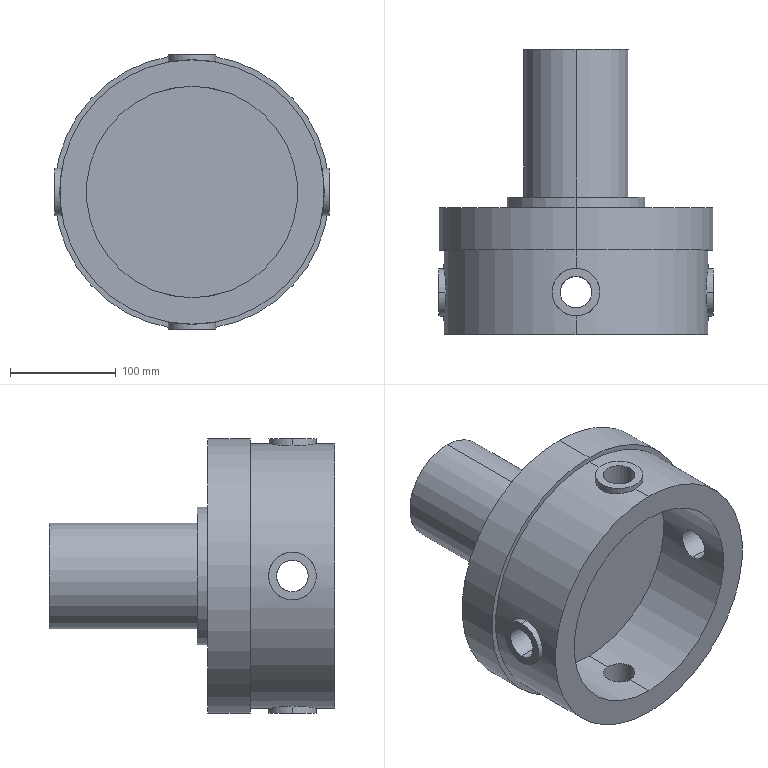Part | SolidWorks | features ICE 5, CirPattern 2, Extrusion 1 | 1 solid | 36 faces | box 260 x 270 x 260 mm | volume 4719185 mm3 | cylinder 26 | plane 10 | commonest cylinder face diameters 30 x8 45 x8 100 x2 130 x2 200 x2 250 x2